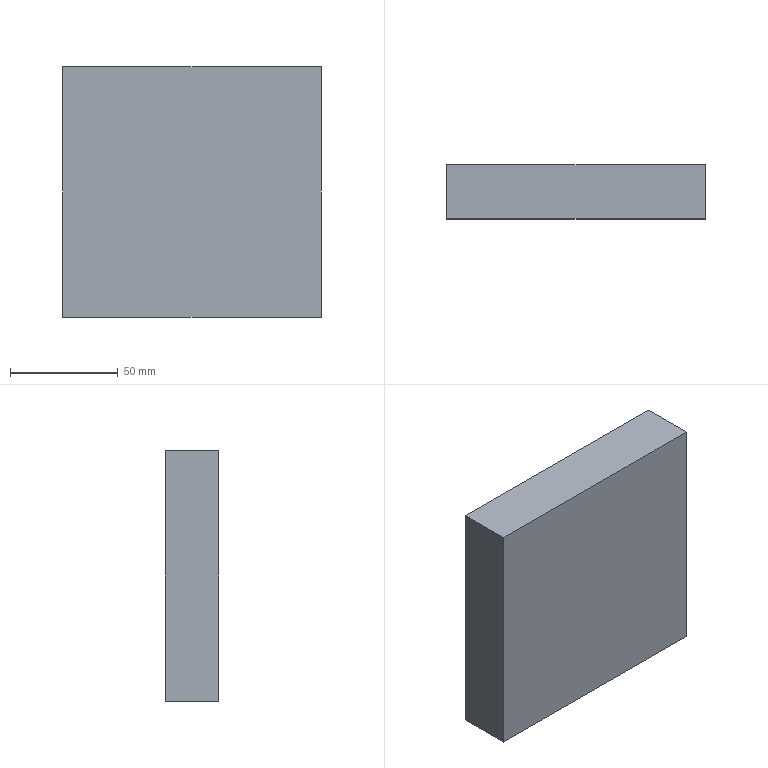Part | NX | features 掩护梁 2 | 1 solid | 8 faces | box 120 x 25 x 116 mm | volume 333863 mm3 | plane 7 | cylinder 1 | commonest cylinder face diameters 30 x1
STEP:
#1=CARTESIAN_POINT('',(-1761.68,3634.947,-172.771));
#2=VERTEX_POINT('',#1);
#3=CARTESIAN_POINT('',(-1761.68,3609.947,-172.771));
#4=VERTEX_POINT('',#3);
#5=CARTESIAN_POINT('',(-1761.68,3634.947,-172.771));
#6=DIRECTION('',(0.,-1.,0.));
#7=VECTOR('',#6,1000.);
#8=LINE('',#5,#7);
#9=EDGE_CURVE('',#2,#4,#8,.T.);
#10=ORIENTED_EDGE('',*,*,#9,.F.);
#11=CARTESIAN_POINT('',(-1761.68,3634.947,-288.771));
#12=VERTEX_POINT('',#11);
#13=CARTESIAN_POINT('',(-1761.68,3634.947,-288.771));
#14=DIRECTION('',(0.,0.,1.));
#15=VECTOR('',#14,1000.);
#16=LINE('',#13,#15);
#17=EDGE_CURVE('',#12,#2,#16,.T.);
#18=ORIENTED_EDGE('',*,*,#17,.F.);
#19=CARTESIAN_POINT('',(-1761.68,3609.947,-288.771));
#20=VERTEX_POINT('',#19);
#21=CARTESIAN_POINT('',(-1761.68,3634.947,-288.771));
#22=DIRECTION('',(0.,-1.,0.));
#23=VECTOR('',#22,1000.);
#24=LINE('',#21,#23);
#25=EDGE_CURVE('',#12,#20,#24,.T.);
#26=ORIENTED_EDGE('',*,*,#25,.T.);
#27=CARTESIAN_POINT('',(-1761.68,3609.947,-288.771));
#28=DIRECTION('',(0.,0.,1.));
#29=VECTOR('',#28,1000.);
#30=LINE('',#27,#29);
#31=EDGE_CURVE('',#20,#4,#30,.T.);
#32=ORIENTED_EDGE('',*,*,#31,.T.);
#33=EDGE_LOOP('',(#10,#18,#26,#32));
#34=FACE_BOUND('',#33,.T.);
#35=CARTESIAN_POINT('',(-1761.68,3634.947,-288.771));
#36=DIRECTION('',(-1.,0.,0.));
#37=DIRECTION('',(0.,0.,1.));
#38=AXIS2_PLACEMENT_3D('',#35,#36,#37);
#39=PLANE('',#38);
#40=ADVANCED_FACE('',(#34),#39,.T.);
#41=CARTESIAN_POINT('',(-1701.68,3634.947,-241.771));
#42=VERTEX_POINT('',#41);
#43=CARTESIAN_POINT('',(-1701.68,3634.947,-256.771));
#44=DIRECTION('',(0.,1.,0.));
#45=DIRECTION('',(0.,0.,1.));
#46=AXIS2_PLACEMENT_3D('',#43,#44,#45);
#47=CIRCLE('',#46,15.);
#48=EDGE_CURVE('',#42,#42,#47,.T.);
#49=ORIENTED_EDGE('',*,*,#48,.F.);
#50=EDGE_LOOP('',(#49));
#51=FACE_BOUND('',#50,.T.);
#52=CARTESIAN_POINT('',(-1641.68,3634.947,-172.771));
#53=VERTEX_POINT('',#52);
#54=CARTESIAN_POINT('',(-1641.68,3634.947,-172.771));
#55=DIRECTION('',(-1.,0.,0.));
#56=VECTOR('',#55,1000.);
#57=LINE('',#54,#56);
#58=EDGE_CURVE('',#53,#2,#57,.T.);
#59=ORIENTED_EDGE('',*,*,#58,.F.);
#60=CARTESIAN_POINT('',(-1641.68,3634.947,-288.771));
#61=VERTEX_POINT('',#60);
#62=CARTESIAN_POINT('',(-1641.68,3634.947,-288.771));
#63=DIRECTION('',(0.,0.,1.));
#64=VECTOR('',#63,1000.);
#65=LINE('',#62,#64);
#66=EDGE_CURVE('',#61,#53,#65,.T.);
#67=ORIENTED_EDGE('',*,*,#66,.F.);
#68=CARTESIAN_POINT('',(-1641.68,3634.947,-288.771));
#69=DIRECTION('',(-1.,0.,0.));
#70=VECTOR('',#69,1000.);
#71=LINE('',#68,#70);
#72=EDGE_CURVE('',#61,#12,#71,.T.);
#73=ORIENTED_EDGE('',*,*,#72,.T.);
#74=ORIENTED_EDGE('',*,*,#17,.T.);
#75=EDGE_LOOP('',(#59,#67,#73,#74));
#76=FACE_BOUND('',#75,.T.);
#77=CARTESIAN_POINT('',(-1641.68,3634.947,-288.771));
#78=DIRECTION('',(0.,1.,0.));
#79=DIRECTION('',(0.,0.,1.));
#80=AXIS2_PLACEMENT_3D('',#77,#78,#79);
#81=PLANE('',#80);
#82=ADVANCED_FACE('',(#51,#76),#81,.T.);
#83=CARTESIAN_POINT('',(-1641.68,3609.947,-172.771));
#84=VERTEX_POINT('',#83);
#85=CARTESIAN_POINT('',(-1641.68,3634.947,-172.771));
#86=DIRECTION('',(0.,1.,0.));
#87=VECTOR('',#86,1000.);
#88=LINE('',#85,#87);
#89=EDGE_CURVE('',#84,#53,#88,.T.);
#90=ORIENTED_EDGE('',*,*,#89,.F.);
#91=CARTESIAN_POINT('',(-1641.68,3609.947,-288.771));
#92=VERTEX_POINT('',#91);
#93=CARTESIAN_POINT('',(-1641.68,3609.947,-288.771));
#94=DIRECTION('',(0.,0.,1.));
#95=VECTOR('',#94,1000.);
#96=LINE('',#93,#95);
#97=EDGE_CURVE('',#92,#84,#96,.T.);
#98=ORIENTED_EDGE('',*,*,#97,.F.);
#99=CARTESIAN_POINT('',(-1641.68,3634.947,-288.771));
#100=DIRECTION('',(0.,1.,0.));
#101=VECTOR('',#100,1000.);
#102=LINE('',#99,#101);
#103=EDGE_CURVE('',#92,#61,#102,.T.);
#104=ORIENTED_EDGE('',*,*,#103,.T.);
#105=ORIENTED_EDGE('',*,*,#66,.T.);
#106=EDGE_LOOP('',(#90,#98,#104,#105));
#107=FACE_BOUND('',#106,.T.);
#108=CARTESIAN_POINT('',(-1641.68,3634.947,-288.771));
#109=DIRECTION('',(1.,0.,0.));
#110=DIRECTION('',(0.,0.,-1.));
#111=AXIS2_PLACEMENT_3D('',#108,#109,#110);
#112=PLANE('',#111);
#113=ADVANCED_FACE('',(#107),#112,.T.);
#114=CARTESIAN_POINT('',(-1641.68,3609.947,-172.771));
#115=DIRECTION('',(1.,0.,0.));
#116=VECTOR('',#115,1000.);
#117=LINE('',#114,#116);
#118=EDGE_CURVE('',#4,#84,#117,.T.);
#119=ORIENTED_EDGE('',*,*,#118,.F.);
#120=ORIENTED_EDGE('',*,*,#31,.F.);
#121=CARTESIAN_POINT('',(-1641.68,3609.947,-288.771));
#122=DIRECTION('',(1.,0.,0.));
#123=VECTOR('',#122,1000.);
#124=LINE('',#121,#123);
#125=EDGE_CURVE('',#20,#92,#124,.T.);
#126=ORIENTED_EDGE('',*,*,#125,.T.);
#127=ORIENTED_EDGE('',*,*,#97,.T.);
#128=EDGE_LOOP('',(#119,#120,#126,#127));
#129=FACE_BOUND('',#128,.T.);
#130=CARTESIAN_POINT('',(-1641.68,3609.947,-288.771));
#131=DIRECTION('',(0.,-1.,0.));
#132=DIRECTION('',(0.,0.,-1.));
#133=AXIS2_PLACEMENT_3D('',#130,#131,#132);
#134=PLANE('',#133);
#135=ADVANCED_FACE('',(#129),#134,.T.);
#136=ORIENTED_EDGE('',*,*,#25,.F.);
#137=ORIENTED_EDGE('',*,*,#72,.F.);
#138=ORIENTED_EDGE('',*,*,#103,.F.);
#139=ORIENTED_EDGE('',*,*,#125,.F.);
#140=EDGE_LOOP('',(#136,#137,#138,#139));
#141=FACE_BOUND('',#140,.T.);
#142=CARTESIAN_POINT('',(-1761.68,3609.947,-288.771));
#143=DIRECTION('',(0.,0.,-1.));
#144=DIRECTION('',(-1.,0.,0.));
#145=AXIS2_PLACEMENT_3D('',#142,#143,#144);
#146=PLANE('',#145);
#147=ADVANCED_FACE('',(#141),#146,.T.);
#148=ORIENTED_EDGE('',*,*,#9,.T.);
#149=ORIENTED_EDGE('',*,*,#118,.T.);
#150=ORIENTED_EDGE('',*,*,#89,.T.);
#151=ORIENTED_EDGE('',*,*,#58,.T.);
#152=EDGE_LOOP('',(#148,#149,#150,#151));
#153=FACE_BOUND('',#152,.T.);
#154=CARTESIAN_POINT('',(-1761.68,3609.947,-172.771));
#155=DIRECTION('',(0.,0.,-1.));
#156=DIRECTION('',(-1.,0.,0.));
#157=AXIS2_PLACEMENT_3D('',#154,#155,#156);
#158=PLANE('',#157);
#159=ADVANCED_FACE('',(#153),#158,.F.);
#160=ORIENTED_EDGE('',*,*,#48,.T.);
#161=EDGE_LOOP('',(#160));
#162=FACE_BOUND('',#161,.T.);
#163=CARTESIAN_POINT('',(-1701.68,3614.947,-241.771));
#164=VERTEX_POINT('',#163);
#165=CARTESIAN_POINT('',(-1701.68,3614.947,-256.771));
#166=DIRECTION('',(0.,1.,0.));
#167=DIRECTION('',(0.,0.,1.));
#168=AXIS2_PLACEMENT_3D('',#165,#166,#167);
#169=CIRCLE('',#168,15.);
#170=EDGE_CURVE('',#164,#164,#169,.T.);
#171=ORIENTED_EDGE('',*,*,#170,.F.);
#172=EDGE_LOOP('',(#171));
#173=FACE_BOUND('',#172,.T.);
#174=CARTESIAN_POINT('',(-1701.68,3614.947,-256.771));
#175=DIRECTION('',(0.,1.,0.));
#176=DIRECTION('',(0.,0.,1.));
#177=AXIS2_PLACEMENT_3D('',#174,#175,#176);
#178=CYLINDRICAL_SURFACE('',#177,15.);
#179=ADVANCED_FACE('',(#162,#173),#178,.F.);
#180=ORIENTED_EDGE('',*,*,#170,.T.);
#181=EDGE_LOOP('',(#180));
#182=FACE_BOUND('',#181,.T.);
#183=CARTESIAN_POINT('',(-1701.68,3614.947,-256.771));
#184=DIRECTION('',(0.,1.,0.));
#185=DIRECTION('',(0.,0.,1.));
#186=AXIS2_PLACEMENT_3D('',#183,#184,#185);
#187=PLANE('',#186);
#188=ADVANCED_FACE('',(#182),#187,.T.);
#189=CLOSED_SHELL('',(#40,#82,#113,#135,#147,#159,#179,#188));
#190=MANIFOLD_SOLID_BREP('',#189);
#191=(LENGTH_UNIT()NAMED_UNIT(*)SI_UNIT(.MILLI.,.METRE.));
#192=UNCERTAINTY_MEASURE_WITH_UNIT(LENGTH_MEASURE(0.00001),#191,'','');
#193=(NAMED_UNIT(*)PLANE_ANGLE_UNIT()SI_UNIT($,.RADIAN.));
#194=(NAMED_UNIT(*)SI_UNIT($,.STERADIAN.)SOLID_ANGLE_UNIT());
#195=(GEOMETRIC_REPRESENTATION_CONTEXT(3)GLOBAL_UNCERTAINTY_ASSIGNED_CONTEXT((#192))GLOBAL_UNIT_ASSIGNED_CONTEXT((#191,#193,#194))REPRESENTATION_CONTEXT('',''));
#196=ADVANCED_BREP_SHAPE_REPRESENTATION('',(#190),#195);